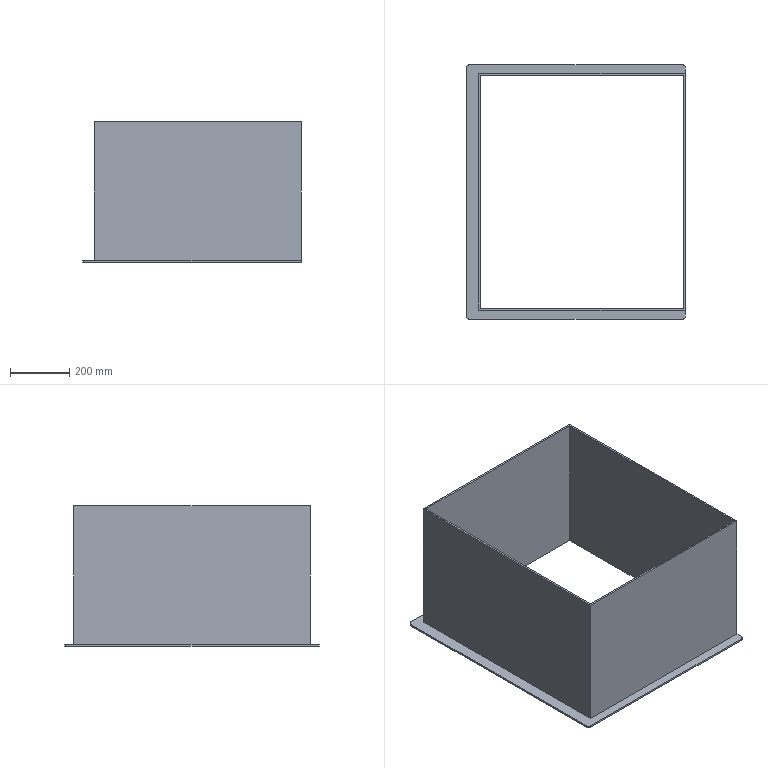Part | STEP file | Maintenance pipe_Default<As machined> | 2 solids | 24 faces | box 740 x 860 x 475 mm | volume 8939485 mm3 | plane 20 | cylinder 4 | commonest cylinder face diameters 20 x4